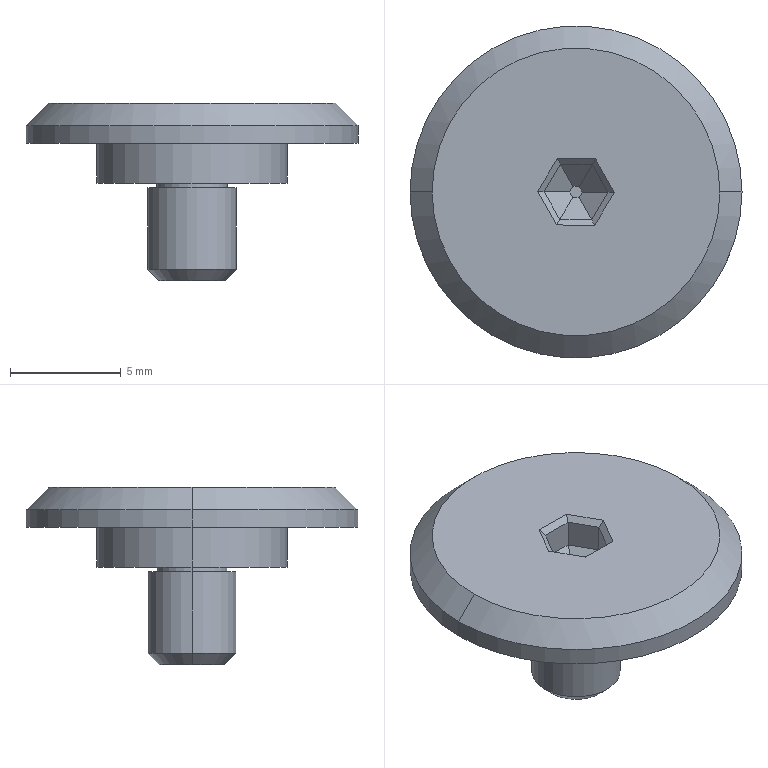Part | NX | features BREP 1 | 1 solid | 36 faces | box 15 x 15 x 8 mm | volume 442.432 mm3 | plane 24 | cylinder 8 | cone 4 | commonest cylinder face diameters 3.2 x2 4 x2 8.6 x2 15 x2
STEP:
#1=CARTESIAN_POINT('',(76.343,184.663,-5.));
#2=VERTEX_POINT('',#1);
#3=CARTESIAN_POINT('',(79.343,184.663,-5.));
#4=VERTEX_POINT('',#3);
#5=CARTESIAN_POINT('',(77.843,184.663,-5.));
#6=DIRECTION('',(0.,0.,-1.));
#7=DIRECTION('',(1.,0.,0.));
#8=AXIS2_PLACEMENT_3D('',#5,#6,#7);
#9=CIRCLE('',#8,1.5);
#10=EDGE_CURVE('',#2,#4,#9,.T.);
#11=ORIENTED_EDGE('',*,*,#10,.F.);
#12=CARTESIAN_POINT('',(75.843,184.663,-4.5));
#13=VERTEX_POINT('',#12);
#14=CARTESIAN_POINT('',(75.843,184.663,-4.5));
#15=DIRECTION('',(-0.7071,0.,0.7071));
#16=VECTOR('',#15,1000.);
#17=LINE('',#14,#16);
#18=EDGE_CURVE('',#2,#13,#17,.T.);
#19=ORIENTED_EDGE('',*,*,#18,.T.);
#20=CARTESIAN_POINT('',(79.843,184.663,-4.5));
#21=VERTEX_POINT('',#20);
#22=CARTESIAN_POINT('',(77.843,184.663,-4.5));
#23=DIRECTION('',(0.,0.,1.));
#24=DIRECTION('',(1.,0.,0.));
#25=AXIS2_PLACEMENT_3D('',#22,#23,#24);
#26=CIRCLE('',#25,2.);
#27=EDGE_CURVE('',#21,#13,#26,.T.);
#28=ORIENTED_EDGE('',*,*,#27,.F.);
#29=CARTESIAN_POINT('',(79.843,184.663,-4.5));
#30=DIRECTION('',(0.7071,0.,0.7071));
#31=VECTOR('',#30,1000.);
#32=LINE('',#29,#31);
#33=EDGE_CURVE('',#4,#21,#32,.T.);
#34=ORIENTED_EDGE('',*,*,#33,.F.);
#35=EDGE_LOOP('',(#11,#19,#28,#34));
#36=FACE_BOUND('',#35,.T.);
#37=CARTESIAN_POINT('',(77.843,184.663,-4.5));
#38=DIRECTION('',(0.,0.,1.));
#39=DIRECTION('',(-1.,0.,0.));
#40=AXIS2_PLACEMENT_3D('',#37,#38,#39);
#41=CONICAL_SURFACE('',#40,2.,0.7854);
#42=ADVANCED_FACE('',(#36),#41,.T.);
#43=ORIENTED_EDGE('',*,*,#27,.T.);
#44=CARTESIAN_POINT('',(75.843,184.663,-0.8));
#45=VERTEX_POINT('',#44);
#46=CARTESIAN_POINT('',(75.843,184.663,-4.));
#47=DIRECTION('',(0.,0.,1.));
#48=VECTOR('',#47,1000.);
#49=LINE('',#46,#48);
#50=EDGE_CURVE('',#13,#45,#49,.T.);
#51=ORIENTED_EDGE('',*,*,#50,.T.);
#52=CARTESIAN_POINT('',(79.843,184.663,-0.8));
#53=VERTEX_POINT('',#52);
#54=CARTESIAN_POINT('',(77.843,184.663,-0.8));
#55=DIRECTION('',(0.,0.,1.));
#56=DIRECTION('',(-1.,0.,0.));
#57=AXIS2_PLACEMENT_3D('',#54,#55,#56);
#58=CIRCLE('',#57,2.);
#59=EDGE_CURVE('',#53,#45,#58,.T.);
#60=ORIENTED_EDGE('',*,*,#59,.F.);
#61=CARTESIAN_POINT('',(79.843,184.663,-4.));
#62=DIRECTION('',(0.,0.,1.));
#63=VECTOR('',#62,1000.);
#64=LINE('',#61,#63);
#65=EDGE_CURVE('',#21,#53,#64,.T.);
#66=ORIENTED_EDGE('',*,*,#65,.F.);
#67=EDGE_LOOP('',(#43,#51,#60,#66));
#68=FACE_BOUND('',#67,.T.);
#69=CARTESIAN_POINT('',(77.843,184.663,-4.));
#70=DIRECTION('',(0.,0.,1.));
#71=DIRECTION('',(-1.,0.,0.));
#72=AXIS2_PLACEMENT_3D('',#69,#70,#71);
#73=CYLINDRICAL_SURFACE('',#72,2.);
#74=ADVANCED_FACE('',(#68),#73,.T.);
#75=CARTESIAN_POINT('',(76.243,184.663,-0.8));
#76=VERTEX_POINT('',#75);
#77=CARTESIAN_POINT('',(79.443,184.663,-0.8));
#78=VERTEX_POINT('',#77);
#79=CARTESIAN_POINT('',(77.843,184.663,-0.8));
#80=DIRECTION('',(0.,0.,-1.));
#81=DIRECTION('',(-1.,0.,0.));
#82=AXIS2_PLACEMENT_3D('',#79,#80,#81);
#83=CIRCLE('',#82,1.6);
#84=EDGE_CURVE('',#76,#78,#83,.T.);
#85=ORIENTED_EDGE('',*,*,#84,.F.);
#86=CARTESIAN_POINT('',(76.243,184.663,-0.6));
#87=VERTEX_POINT('',#86);
#88=CARTESIAN_POINT('',(76.243,184.663,-0.8));
#89=DIRECTION('',(0.,0.,1.));
#90=VECTOR('',#89,1000.);
#91=LINE('',#88,#90);
#92=EDGE_CURVE('',#76,#87,#91,.T.);
#93=ORIENTED_EDGE('',*,*,#92,.T.);
#94=CARTESIAN_POINT('',(79.443,184.663,-0.6));
#95=VERTEX_POINT('',#94);
#96=CARTESIAN_POINT('',(77.843,184.663,-0.6));
#97=DIRECTION('',(0.,0.,-1.));
#98=DIRECTION('',(1.,0.,0.));
#99=AXIS2_PLACEMENT_3D('',#96,#97,#98);
#100=CIRCLE('',#99,1.6);
#101=EDGE_CURVE('',#87,#95,#100,.T.);
#102=ORIENTED_EDGE('',*,*,#101,.T.);
#103=CARTESIAN_POINT('',(79.443,184.663,-0.8));
#104=DIRECTION('',(0.,0.,1.));
#105=VECTOR('',#104,1000.);
#106=LINE('',#103,#105);
#107=EDGE_CURVE('',#78,#95,#106,.T.);
#108=ORIENTED_EDGE('',*,*,#107,.F.);
#109=EDGE_LOOP('',(#85,#93,#102,#108));
#110=FACE_BOUND('',#109,.T.);
#111=CARTESIAN_POINT('',(77.843,184.663,-0.8));
#112=DIRECTION('',(0.,0.,1.));
#113=DIRECTION('',(-1.,0.,0.));
#114=AXIS2_PLACEMENT_3D('',#111,#112,#113);
#115=CYLINDRICAL_SURFACE('',#114,1.6);
#116=ADVANCED_FACE('',(#110),#115,.T.);
#117=CARTESIAN_POINT('',(84.343,184.663,3.));
#118=VERTEX_POINT('',#117);
#119=CARTESIAN_POINT('',(71.343,184.663,3.));
#120=VERTEX_POINT('',#119);
#121=CARTESIAN_POINT('',(77.843,184.663,3.));
#122=DIRECTION('',(0.,0.,1.));
#123=DIRECTION('',(1.,0.,0.));
#124=AXIS2_PLACEMENT_3D('',#121,#122,#123);
#125=CIRCLE('',#124,6.5);
#126=EDGE_CURVE('',#118,#120,#125,.T.);
#127=ORIENTED_EDGE('',*,*,#126,.F.);
#128=CARTESIAN_POINT('',(85.343,184.663,2.));
#129=VERTEX_POINT('',#128);
#130=CARTESIAN_POINT('',(84.343,184.663,3.));
#131=DIRECTION('',(0.7071,0.,-0.7071));
#132=VECTOR('',#131,1000.);
#133=LINE('',#130,#132);
#134=EDGE_CURVE('',#129,#118,#133,.F.);
#135=ORIENTED_EDGE('',*,*,#134,.F.);
#136=CARTESIAN_POINT('',(70.343,184.663,2.));
#137=VERTEX_POINT('',#136);
#138=CARTESIAN_POINT('',(77.843,184.663,2.));
#139=DIRECTION('',(0.,0.,-1.));
#140=DIRECTION('',(1.,0.,0.));
#141=AXIS2_PLACEMENT_3D('',#138,#139,#140);
#142=CIRCLE('',#141,7.5);
#143=EDGE_CURVE('',#137,#129,#142,.T.);
#144=ORIENTED_EDGE('',*,*,#143,.F.);
#145=CARTESIAN_POINT('',(71.343,184.663,3.));
#146=DIRECTION('',(-0.7071,0.,-0.7071));
#147=VECTOR('',#146,1000.);
#148=LINE('',#145,#147);
#149=EDGE_CURVE('',#137,#120,#148,.F.);
#150=ORIENTED_EDGE('',*,*,#149,.T.);
#151=EDGE_LOOP('',(#127,#135,#144,#150));
#152=FACE_BOUND('',#151,.T.);
#153=CARTESIAN_POINT('',(77.843,184.663,3.));
#154=DIRECTION('',(0.,0.,-1.));
#155=DIRECTION('',(1.,0.,0.));
#156=AXIS2_PLACEMENT_3D('',#153,#154,#155);
#157=CONICAL_SURFACE('',#156,6.5,0.7854);
#158=ADVANCED_FACE('',(#152),#157,.T.);
#159=ORIENTED_EDGE('',*,*,#143,.T.);
#160=CARTESIAN_POINT('',(85.343,184.663,1.2));
#161=VERTEX_POINT('',#160);
#162=CARTESIAN_POINT('',(85.343,184.663,2.));
#163=DIRECTION('',(0.,0.,-1.));
#164=VECTOR('',#163,1000.);
#165=LINE('',#162,#164);
#166=EDGE_CURVE('',#161,#129,#165,.F.);
#167=ORIENTED_EDGE('',*,*,#166,.F.);
#168=CARTESIAN_POINT('',(70.343,184.663,1.2));
#169=VERTEX_POINT('',#168);
#170=CARTESIAN_POINT('',(77.843,184.663,1.2));
#171=DIRECTION('',(0.,0.,1.));
#172=DIRECTION('',(1.,0.,0.));
#173=AXIS2_PLACEMENT_3D('',#170,#171,#172);
#174=CIRCLE('',#173,7.5);
#175=EDGE_CURVE('',#161,#169,#174,.T.);
#176=ORIENTED_EDGE('',*,*,#175,.T.);
#177=CARTESIAN_POINT('',(70.343,184.663,2.));
#178=DIRECTION('',(0.,0.,-1.));
#179=VECTOR('',#178,1000.);
#180=LINE('',#177,#179);
#181=EDGE_CURVE('',#169,#137,#180,.F.);
#182=ORIENTED_EDGE('',*,*,#181,.T.);
#183=EDGE_LOOP('',(#159,#167,#176,#182));
#184=FACE_BOUND('',#183,.T.);
#185=CARTESIAN_POINT('',(77.843,184.663,2.));
#186=DIRECTION('',(0.,0.,-1.));
#187=DIRECTION('',(1.,0.,0.));
#188=AXIS2_PLACEMENT_3D('',#185,#186,#187);
#189=CYLINDRICAL_SURFACE('',#188,7.5);
#190=ADVANCED_FACE('',(#184),#189,.T.);
#191=CARTESIAN_POINT('',(82.143,184.663,1.2));
#192=VERTEX_POINT('',#191);
#193=CARTESIAN_POINT('',(73.543,184.663,1.2));
#194=VERTEX_POINT('',#193);
#195=CARTESIAN_POINT('',(77.843,184.663,1.2));
#196=DIRECTION('',(0.,0.,1.));
#197=DIRECTION('',(1.,0.,0.));
#198=AXIS2_PLACEMENT_3D('',#195,#196,#197);
#199=CIRCLE('',#198,4.3);
#200=EDGE_CURVE('',#192,#194,#199,.T.);
#201=ORIENTED_EDGE('',*,*,#200,.F.);
#202=CARTESIAN_POINT('',(82.143,184.663,-0.6));
#203=VERTEX_POINT('',#202);
#204=CARTESIAN_POINT('',(82.143,184.663,1.));
#205=DIRECTION('',(0.,0.,-1.));
#206=VECTOR('',#205,1000.);
#207=LINE('',#204,#206);
#208=EDGE_CURVE('',#203,#192,#207,.F.);
#209=ORIENTED_EDGE('',*,*,#208,.F.);
#210=CARTESIAN_POINT('',(73.543,184.663,-0.6));
#211=VERTEX_POINT('',#210);
#212=CARTESIAN_POINT('',(77.843,184.663,-0.6));
#213=DIRECTION('',(0.,0.,1.));
#214=DIRECTION('',(1.,0.,0.));
#215=AXIS2_PLACEMENT_3D('',#212,#213,#214);
#216=CIRCLE('',#215,4.3);
#217=EDGE_CURVE('',#203,#211,#216,.T.);
#218=ORIENTED_EDGE('',*,*,#217,.T.);
#219=CARTESIAN_POINT('',(73.543,184.663,1.));
#220=DIRECTION('',(0.,0.,-1.));
#221=VECTOR('',#220,1000.);
#222=LINE('',#219,#221);
#223=EDGE_CURVE('',#211,#194,#222,.F.);
#224=ORIENTED_EDGE('',*,*,#223,.T.);
#225=EDGE_LOOP('',(#201,#209,#218,#224));
#226=FACE_BOUND('',#225,.T.);
#227=CARTESIAN_POINT('',(77.843,184.663,1.));
#228=DIRECTION('',(0.,0.,-1.));
#229=DIRECTION('',(1.,0.,0.));
#230=AXIS2_PLACEMENT_3D('',#227,#228,#229);
#231=CYLINDRICAL_SURFACE('',#230,4.3);
#232=ADVANCED_FACE('',(#226),#231,.T.);
#233=ORIENTED_EDGE('',*,*,#208,.T.);
#234=CARTESIAN_POINT('',(77.843,184.663,1.2));
#235=DIRECTION('',(0.,0.,1.));
#236=DIRECTION('',(1.,0.,0.));
#237=AXIS2_PLACEMENT_3D('',#234,#235,#236);
#238=CIRCLE('',#237,4.3);
#239=EDGE_CURVE('',#194,#192,#238,.T.);
#240=ORIENTED_EDGE('',*,*,#239,.F.);
#241=ORIENTED_EDGE('',*,*,#223,.F.);
#242=CARTESIAN_POINT('',(77.843,184.663,-0.6));
#243=DIRECTION('',(0.,0.,1.));
#244=DIRECTION('',(1.,0.,0.));
#245=AXIS2_PLACEMENT_3D('',#242,#243,#244);
#246=CIRCLE('',#245,4.3);
#247=EDGE_CURVE('',#211,#203,#246,.T.);
#248=ORIENTED_EDGE('',*,*,#247,.T.);
#249=EDGE_LOOP('',(#233,#240,#241,#248));
#250=FACE_BOUND('',#249,.T.);
#251=CARTESIAN_POINT('',(77.843,184.663,1.));
#252=DIRECTION('',(0.,0.,-1.));
#253=DIRECTION('',(1.,0.,0.));
#254=AXIS2_PLACEMENT_3D('',#251,#252,#253);
#255=CYLINDRICAL_SURFACE('',#254,4.3);
#256=ADVANCED_FACE('',(#250),#255,.T.);
#257=ORIENTED_EDGE('',*,*,#247,.F.);
#258=ORIENTED_EDGE('',*,*,#217,.F.);
#259=EDGE_LOOP('',(#257,#258));
#260=FACE_BOUND('',#259,.T.);
#261=CARTESIAN_POINT('',(77.843,184.663,-0.6));
#262=DIRECTION('',(0.,0.,-1.));
#263=DIRECTION('',(1.,0.,0.));
#264=AXIS2_PLACEMENT_3D('',#261,#262,#263);
#265=CIRCLE('',#264,1.6);
#266=EDGE_CURVE('',#95,#87,#265,.T.);
#267=ORIENTED_EDGE('',*,*,#266,.F.);
#268=ORIENTED_EDGE('',*,*,#101,.F.);
#269=EDGE_LOOP('',(#267,#268));
#270=FACE_BOUND('',#269,.T.);
#271=CARTESIAN_POINT('',(77.843,184.663,-0.6));
#272=DIRECTION('',(0.,0.,1.));
#273=DIRECTION('',(-1.,0.,0.));
#274=AXIS2_PLACEMENT_3D('',#271,#272,#273);
#275=PLANE('',#274);
#276=ADVANCED_FACE('',(#260,#270),#275,.F.);
#277=ORIENTED_EDGE('',*,*,#166,.T.);
#278=CARTESIAN_POINT('',(77.843,184.663,2.));
#279=DIRECTION('',(0.,0.,-1.));
#280=DIRECTION('',(1.,0.,0.));
#281=AXIS2_PLACEMENT_3D('',#278,#279,#280);
#282=CIRCLE('',#281,7.5);
#283=EDGE_CURVE('',#129,#137,#282,.T.);
#284=ORIENTED_EDGE('',*,*,#283,.T.);
#285=ORIENTED_EDGE('',*,*,#181,.F.);
#286=CARTESIAN_POINT('',(77.843,184.663,1.2));
#287=DIRECTION('',(0.,0.,1.));
#288=DIRECTION('',(1.,0.,0.));
#289=AXIS2_PLACEMENT_3D('',#286,#287,#288);
#290=CIRCLE('',#289,7.5);
#291=EDGE_CURVE('',#169,#161,#290,.T.);
#292=ORIENTED_EDGE('',*,*,#291,.T.);
#293=EDGE_LOOP('',(#277,#284,#285,#292));
#294=FACE_BOUND('',#293,.T.);
#295=CARTESIAN_POINT('',(77.843,184.663,2.));
#296=DIRECTION('',(0.,0.,-1.));
#297=DIRECTION('',(1.,0.,0.));
#298=AXIS2_PLACEMENT_3D('',#295,#296,#297);
#299=CYLINDRICAL_SURFACE('',#298,7.5);
#300=ADVANCED_FACE('',(#294),#299,.T.);
#301=CARTESIAN_POINT('',(77.843,184.663,3.));
#302=DIRECTION('',(0.,0.,1.));
#303=DIRECTION('',(1.,0.,0.));
#304=AXIS2_PLACEMENT_3D('',#301,#302,#303);
#305=CIRCLE('',#304,6.5);
#306=EDGE_CURVE('',#120,#118,#305,.T.);
#307=ORIENTED_EDGE('',*,*,#306,.T.);
#308=ORIENTED_EDGE('',*,*,#126,.T.);
#309=EDGE_LOOP('',(#307,#308));
#310=FACE_BOUND('',#309,.T.);
#311=CARTESIAN_POINT('',(76.111,184.683,3.));
#312=VERTEX_POINT('',#311);
#313=CARTESIAN_POINT('',(76.995,186.173,3.));
#314=VERTEX_POINT('',#313);
#315=CARTESIAN_POINT('',(76.921,186.049,3.));
#316=DIRECTION('',(0.5101,0.8601,0.));
#317=VECTOR('',#316,1000.);
#318=LINE('',#315,#317);
#319=EDGE_CURVE('',#312,#314,#318,.T.);
#320=ORIENTED_EDGE('',*,*,#319,.T.);
#321=CARTESIAN_POINT('',(78.727,186.152,3.));
#322=VERTEX_POINT('',#321);
#323=CARTESIAN_POINT('',(78.582,186.154,3.));
#324=DIRECTION('',(0.9999,-0.01175,0.));
#325=VECTOR('',#324,1000.);
#326=LINE('',#323,#325);
#327=EDGE_CURVE('',#314,#322,#326,.T.);
#328=ORIENTED_EDGE('',*,*,#327,.T.);
#329=CARTESIAN_POINT('',(79.575,184.642,3.));
#330=VERTEX_POINT('',#329);
#331=CARTESIAN_POINT('',(79.504,184.768,3.));
#332=DIRECTION('',(0.4898,-0.8718,0.));
#333=VECTOR('',#332,1000.);
#334=LINE('',#331,#333);
#335=EDGE_CURVE('',#322,#330,#334,.T.);
#336=ORIENTED_EDGE('',*,*,#335,.T.);
#337=CARTESIAN_POINT('',(78.691,183.153,3.));
#338=VERTEX_POINT('',#337);
#339=CARTESIAN_POINT('',(78.765,183.277,3.));
#340=DIRECTION('',(-0.5101,-0.8601,0.));
#341=VECTOR('',#340,1000.);
#342=LINE('',#339,#341);
#343=EDGE_CURVE('',#330,#338,#342,.T.);
#344=ORIENTED_EDGE('',*,*,#343,.T.);
#345=CARTESIAN_POINT('',(76.96,183.173,3.));
#346=VERTEX_POINT('',#345);
#347=CARTESIAN_POINT('',(77.104,183.171,3.));
#348=DIRECTION('',(-0.9999,0.01175,0.));
#349=VECTOR('',#348,1000.);
#350=LINE('',#347,#349);
#351=EDGE_CURVE('',#338,#346,#350,.T.);
#352=ORIENTED_EDGE('',*,*,#351,.T.);
#353=CARTESIAN_POINT('',(76.182,184.557,3.));
#354=DIRECTION('',(-0.4898,0.8718,0.));
#355=VECTOR('',#354,1000.);
#356=LINE('',#353,#355);
#357=EDGE_CURVE('',#346,#312,#356,.T.);
#358=ORIENTED_EDGE('',*,*,#357,.T.);
#359=EDGE_LOOP('',(#320,#328,#336,#344,#352,#358));
#360=FACE_BOUND('',#359,.T.);
#361=CARTESIAN_POINT('',(77.843,184.663,3.));
#362=DIRECTION('',(0.,0.,1.));
#363=DIRECTION('',(-1.,0.,0.));
#364=AXIS2_PLACEMENT_3D('',#361,#362,#363);
#365=PLANE('',#364);
#366=ADVANCED_FACE('',(#310,#360),#365,.T.);
#367=ORIENTED_EDGE('',*,*,#291,.F.);
#368=ORIENTED_EDGE('',*,*,#175,.F.);
#369=EDGE_LOOP('',(#367,#368));
#370=FACE_BOUND('',#369,.T.);
#371=ORIENTED_EDGE('',*,*,#239,.T.);
#372=ORIENTED_EDGE('',*,*,#200,.T.);
#373=EDGE_LOOP('',(#371,#372));
#374=FACE_BOUND('',#373,.T.);
#375=CARTESIAN_POINT('',(77.843,184.663,1.2));
#376=DIRECTION('',(0.,0.,1.));
#377=DIRECTION('',(-1.,0.,0.));
#378=AXIS2_PLACEMENT_3D('',#375,#376,#377);
#379=PLANE('',#378);
#380=ADVANCED_FACE('',(#370,#374),#379,.F.);
#381=CARTESIAN_POINT('',(79.286,184.646,1.5));
#382=VERTEX_POINT('',#381);
#383=CARTESIAN_POINT('',(79.286,184.646,2.75));
#384=VERTEX_POINT('',#383);
#385=CARTESIAN_POINT('',(79.286,184.646,1.5));
#386=DIRECTION('',(0.,0.,1.));
#387=VECTOR('',#386,1000.);
#388=LINE('',#385,#387);
#389=EDGE_CURVE('',#382,#384,#388,.T.);
#390=ORIENTED_EDGE('',*,*,#389,.T.);
#391=CARTESIAN_POINT('',(78.579,185.904,2.75));
#392=VERTEX_POINT('',#391);
#393=CARTESIAN_POINT('',(78.579,185.904,2.75));
#394=DIRECTION('',(-0.4898,0.8718,0.));
#395=VECTOR('',#394,1000.);
#396=LINE('',#393,#395);
#397=EDGE_CURVE('',#384,#392,#396,.T.);
#398=ORIENTED_EDGE('',*,*,#397,.T.);
#399=CARTESIAN_POINT('',(78.579,185.904,1.5));
#400=VERTEX_POINT('',#399);
#401=CARTESIAN_POINT('',(78.579,185.904,1.5));
#402=DIRECTION('',(0.,0.,1.));
#403=VECTOR('',#402,1000.);
#404=LINE('',#401,#403);
#405=EDGE_CURVE('',#400,#392,#404,.T.);
#406=ORIENTED_EDGE('',*,*,#405,.F.);
#407=CARTESIAN_POINT('',(79.286,184.646,1.5));
#408=DIRECTION('',(-0.4898,0.8718,0.));
#409=VECTOR('',#408,1000.);
#410=LINE('',#407,#409);
#411=EDGE_CURVE('',#382,#400,#410,.T.);
#412=ORIENTED_EDGE('',*,*,#411,.F.);
#413=EDGE_LOOP('',(#390,#398,#406,#412));
#414=FACE_BOUND('',#413,.T.);
#415=CARTESIAN_POINT('',(79.286,184.646,1.5));
#416=DIRECTION('',(0.8718,0.4898,0.));
#417=DIRECTION('',(0.,0.,1.));
#418=AXIS2_PLACEMENT_3D('',#415,#416,#417);
#419=PLANE('',#418);
#420=ADVANCED_FACE('',(#414),#419,.F.);
#421=CARTESIAN_POINT('',(78.55,183.404,1.5));
#422=VERTEX_POINT('',#421);
#423=CARTESIAN_POINT('',(78.55,183.404,2.75));
#424=VERTEX_POINT('',#423);
#425=CARTESIAN_POINT('',(78.55,183.404,1.5));
#426=DIRECTION('',(0.,0.,1.));
#427=VECTOR('',#426,1000.);
#428=LINE('',#425,#427);
#429=EDGE_CURVE('',#422,#424,#428,.T.);
#430=ORIENTED_EDGE('',*,*,#429,.T.);
#431=CARTESIAN_POINT('',(79.286,184.646,2.75));
#432=DIRECTION('',(0.5101,0.8601,0.));
#433=VECTOR('',#432,1000.);
#434=LINE('',#431,#433);
#435=EDGE_CURVE('',#424,#384,#434,.T.);
#436=ORIENTED_EDGE('',*,*,#435,.T.);
#437=ORIENTED_EDGE('',*,*,#389,.F.);
#438=CARTESIAN_POINT('',(78.55,183.404,1.5));
#439=DIRECTION('',(0.5101,0.8601,0.));
#440=VECTOR('',#439,1000.);
#441=LINE('',#438,#440);
#442=EDGE_CURVE('',#422,#382,#441,.T.);
#443=ORIENTED_EDGE('',*,*,#442,.F.);
#444=EDGE_LOOP('',(#430,#436,#437,#443));
#445=FACE_BOUND('',#444,.T.);
#446=CARTESIAN_POINT('',(78.55,183.404,1.5));
#447=DIRECTION('',(0.8601,-0.5101,0.));
#448=DIRECTION('',(0.,0.,1.));
#449=AXIS2_PLACEMENT_3D('',#446,#447,#448);
#450=PLANE('',#449);
#451=ADVANCED_FACE('',(#445),#450,.F.);
#452=CARTESIAN_POINT('',(77.107,183.421,1.5));
#453=VERTEX_POINT('',#452);
#454=CARTESIAN_POINT('',(77.107,183.421,2.75));
#455=VERTEX_POINT('',#454);
#456=CARTESIAN_POINT('',(77.107,183.421,1.5));
#457=DIRECTION('',(0.,0.,1.));
#458=VECTOR('',#457,1000.);
#459=LINE('',#456,#458);
#460=EDGE_CURVE('',#453,#455,#459,.T.);
#461=ORIENTED_EDGE('',*,*,#460,.T.);
#462=CARTESIAN_POINT('',(78.55,183.404,2.75));
#463=DIRECTION('',(0.9999,-0.01175,0.));
#464=VECTOR('',#463,1000.);
#465=LINE('',#462,#464);
#466=EDGE_CURVE('',#455,#424,#465,.T.);
#467=ORIENTED_EDGE('',*,*,#466,.T.);
#468=ORIENTED_EDGE('',*,*,#429,.F.);
#469=CARTESIAN_POINT('',(77.107,183.421,1.5));
#470=DIRECTION('',(0.9999,-0.01175,0.));
#471=VECTOR('',#470,1000.);
#472=LINE('',#469,#471);
#473=EDGE_CURVE('',#453,#422,#472,.T.);
#474=ORIENTED_EDGE('',*,*,#473,.F.);
#475=EDGE_LOOP('',(#461,#467,#468,#474));
#476=FACE_BOUND('',#475,.T.);
#477=CARTESIAN_POINT('',(77.107,183.421,1.5));
#478=DIRECTION('',(-0.01175,-0.9999,0.));
#479=DIRECTION('',(0.9999,-0.01175,0.));
#480=AXIS2_PLACEMENT_3D('',#477,#478,#479);
#481=PLANE('',#480);
#482=ADVANCED_FACE('',(#476),#481,.F.);
#483=CARTESIAN_POINT('',(76.4,184.68,1.5));
#484=VERTEX_POINT('',#483);
#485=CARTESIAN_POINT('',(76.4,184.68,2.75));
#486=VERTEX_POINT('',#485);
#487=CARTESIAN_POINT('',(76.4,184.68,1.5));
#488=DIRECTION('',(0.,0.,1.));
#489=VECTOR('',#488,1000.);
#490=LINE('',#487,#489);
#491=EDGE_CURVE('',#484,#486,#490,.T.);
#492=ORIENTED_EDGE('',*,*,#491,.T.);
#493=CARTESIAN_POINT('',(77.107,183.421,2.75));
#494=DIRECTION('',(0.4898,-0.8718,0.));
#495=VECTOR('',#494,1000.);
#496=LINE('',#493,#495);
#497=EDGE_CURVE('',#486,#455,#496,.T.);
#498=ORIENTED_EDGE('',*,*,#497,.T.);
#499=ORIENTED_EDGE('',*,*,#460,.F.);
#500=CARTESIAN_POINT('',(76.4,184.68,1.5));
#501=DIRECTION('',(0.4898,-0.8718,0.));
#502=VECTOR('',#501,1000.);
#503=LINE('',#500,#502);
#504=EDGE_CURVE('',#484,#453,#503,.T.);
#505=ORIENTED_EDGE('',*,*,#504,.F.);
#506=EDGE_LOOP('',(#492,#498,#499,#505));
#507=FACE_BOUND('',#506,.T.);
#508=CARTESIAN_POINT('',(76.4,184.68,1.5));
#509=DIRECTION('',(-0.8718,-0.4898,0.));
#510=DIRECTION('',(0.4898,-0.8718,0.));
#511=AXIS2_PLACEMENT_3D('',#508,#509,#510);
#512=PLANE('',#511);
#513=ADVANCED_FACE('',(#507),#512,.F.);
#514=CARTESIAN_POINT('',(77.136,185.921,1.5));
#515=VERTEX_POINT('',#514);
#516=CARTESIAN_POINT('',(77.136,185.921,2.75));
#517=VERTEX_POINT('',#516);
#518=CARTESIAN_POINT('',(77.136,185.921,1.5));
#519=DIRECTION('',(0.,0.,1.));
#520=VECTOR('',#519,1000.);
#521=LINE('',#518,#520);
#522=EDGE_CURVE('',#515,#517,#521,.T.);
#523=ORIENTED_EDGE('',*,*,#522,.T.);
#524=CARTESIAN_POINT('',(76.4,184.68,2.75));
#525=DIRECTION('',(-0.5101,-0.8601,0.));
#526=VECTOR('',#525,1000.);
#527=LINE('',#524,#526);
#528=EDGE_CURVE('',#517,#486,#527,.T.);
#529=ORIENTED_EDGE('',*,*,#528,.T.);
#530=ORIENTED_EDGE('',*,*,#491,.F.);
#531=CARTESIAN_POINT('',(77.136,185.921,1.5));
#532=DIRECTION('',(-0.5101,-0.8601,0.));
#533=VECTOR('',#532,1000.);
#534=LINE('',#531,#533);
#535=EDGE_CURVE('',#515,#484,#534,.T.);
#536=ORIENTED_EDGE('',*,*,#535,.F.);
#537=EDGE_LOOP('',(#523,#529,#530,#536));
#538=FACE_BOUND('',#537,.T.);
#539=CARTESIAN_POINT('',(77.136,185.921,1.5));
#540=DIRECTION('',(-0.8601,0.5101,0.));
#541=DIRECTION('',(0.,0.,-1.));
#542=AXIS2_PLACEMENT_3D('',#539,#540,#541);
#543=PLANE('',#542);
#544=ADVANCED_FACE('',(#538),#543,.F.);
#545=ORIENTED_EDGE('',*,*,#405,.T.);
#546=CARTESIAN_POINT('',(77.136,185.921,2.75));
#547=DIRECTION('',(-0.9999,0.01175,0.));
#548=VECTOR('',#547,1000.);
#549=LINE('',#546,#548);
#550=EDGE_CURVE('',#392,#517,#549,.T.);
#551=ORIENTED_EDGE('',*,*,#550,.T.);
#552=ORIENTED_EDGE('',*,*,#522,.F.);
#553=CARTESIAN_POINT('',(78.579,185.904,1.5));
#554=DIRECTION('',(-0.9999,0.01175,0.));
#555=VECTOR('',#554,1000.);
#556=LINE('',#553,#555);
#557=EDGE_CURVE('',#400,#515,#556,.T.);
#558=ORIENTED_EDGE('',*,*,#557,.F.);
#559=EDGE_LOOP('',(#545,#551,#552,#558));
#560=FACE_BOUND('',#559,.T.);
#561=CARTESIAN_POINT('',(78.579,185.904,1.5));
#562=DIRECTION('',(0.01175,0.9999,0.));
#563=DIRECTION('',(0.,0.,1.));
#564=AXIS2_PLACEMENT_3D('',#561,#562,#563);
#565=PLANE('',#564);
#566=ADVANCED_FACE('',(#560),#565,.F.);
#567=ORIENTED_EDGE('',*,*,#442,.T.);
#568=CARTESIAN_POINT('',(78.132,184.659,0.5));
#569=VERTEX_POINT('',#568);
#570=CARTESIAN_POINT('',(78.874,184.651,1.143));
#571=DIRECTION('',(0.7559,-0.008884,0.6547));
#572=VECTOR('',#571,1000.);
#573=LINE('',#570,#572);
#574=EDGE_CURVE('',#569,#382,#573,.T.);
#575=ORIENTED_EDGE('',*,*,#574,.F.);
#576=CARTESIAN_POINT('',(77.984,184.411,0.5));
#577=VERTEX_POINT('',#576);
#578=CARTESIAN_POINT('',(-23.225,13.775,0.5));
#579=DIRECTION('',(0.5101,0.8601,0.));
#580=VECTOR('',#579,1000.);
#581=LINE('',#578,#580);
#582=EDGE_CURVE('',#577,#569,#581,.T.);
#583=ORIENTED_EDGE('',*,*,#582,.F.);
#584=CARTESIAN_POINT('',(78.348,183.764,1.143));
#585=DIRECTION('',(0.3702,-0.6591,0.6547));
#586=VECTOR('',#585,1000.);
#587=LINE('',#584,#586);
#588=EDGE_CURVE('',#577,#422,#587,.T.);
#589=ORIENTED_EDGE('',*,*,#588,.T.);
#590=EDGE_LOOP('',(#567,#575,#583,#589));
#591=FACE_BOUND('',#590,.T.);
#592=CARTESIAN_POINT('',(78.55,183.404,1.5));
#593=DIRECTION('',(0.6082,-0.3607,-0.7071));
#594=DIRECTION('',(0.,0.8908,-0.4544));
#595=AXIS2_PLACEMENT_3D('',#592,#593,#594);
#596=PLANE('',#595);
#597=ADVANCED_FACE('',(#591),#596,.F.);
#598=ORIENTED_EDGE('',*,*,#473,.T.);
#599=ORIENTED_EDGE('',*,*,#588,.F.);
#600=CARTESIAN_POINT('',(77.696,184.414,0.5));
#601=VERTEX_POINT('',#600);
#602=CARTESIAN_POINT('',(2.178,185.302,0.5));
#603=DIRECTION('',(0.9999,-0.01175,0.));
#604=VECTOR('',#603,1000.);
#605=LINE('',#602,#604);
#606=EDGE_CURVE('',#601,#577,#605,.T.);
#607=ORIENTED_EDGE('',*,*,#606,.F.);
#608=CARTESIAN_POINT('',(77.317,183.776,1.143));
#609=DIRECTION('',(-0.3856,-0.6502,0.6547));
#610=VECTOR('',#609,1000.);
#611=LINE('',#608,#610);
#612=EDGE_CURVE('',#601,#453,#611,.T.);
#613=ORIENTED_EDGE('',*,*,#612,.T.);
#614=EDGE_LOOP('',(#598,#599,#607,#613));
#615=FACE_BOUND('',#614,.T.);
#616=CARTESIAN_POINT('',(77.107,183.421,1.5));
#617=DIRECTION('',(-0.008311,-0.7071,-0.7071));
#618=DIRECTION('',(0.,0.7071,-0.7071));
#619=AXIS2_PLACEMENT_3D('',#616,#617,#618);
#620=PLANE('',#619);
#621=ADVANCED_FACE('',(#615),#620,.F.);
#622=ORIENTED_EDGE('',*,*,#504,.T.);
#623=ORIENTED_EDGE('',*,*,#612,.F.);
#624=CARTESIAN_POINT('',(77.554,184.666,0.5));
#625=VERTEX_POINT('',#624);
#626=CARTESIAN_POINT('',(137.805,77.417,0.5));
#627=DIRECTION('',(0.4898,-0.8718,0.));
#628=VECTOR('',#627,1000.);
#629=LINE('',#626,#628);
#630=EDGE_CURVE('',#625,#601,#629,.T.);
#631=ORIENTED_EDGE('',*,*,#630,.F.);
#632=CARTESIAN_POINT('',(76.812,184.675,1.143));
#633=DIRECTION('',(-0.7559,0.008884,0.6547));
#634=VECTOR('',#633,1000.);
#635=LINE('',#632,#634);
#636=EDGE_CURVE('',#625,#484,#635,.T.);
#637=ORIENTED_EDGE('',*,*,#636,.T.);
#638=EDGE_LOOP('',(#622,#623,#631,#637));
#639=FACE_BOUND('',#638,.T.);
#640=CARTESIAN_POINT('',(76.4,184.68,1.5));
#641=DIRECTION('',(-0.6165,-0.3463,-0.7071));
#642=DIRECTION('',(0.7538,0.,-0.6572));
#643=AXIS2_PLACEMENT_3D('',#640,#641,#642);
#644=PLANE('',#643);
#645=ADVANCED_FACE('',(#639),#644,.F.);
#646=ORIENTED_EDGE('',*,*,#535,.T.);
#647=ORIENTED_EDGE('',*,*,#636,.F.);
#648=CARTESIAN_POINT('',(77.702,184.914,0.5));
#649=VERTEX_POINT('',#648);
#650=CARTESIAN_POINT('',(-23.655,14.03,0.5));
#651=DIRECTION('',(-0.5101,-0.8601,0.));
#652=VECTOR('',#651,1000.);
#653=LINE('',#650,#652);
#654=EDGE_CURVE('',#649,#625,#653,.T.);
#655=ORIENTED_EDGE('',*,*,#654,.F.);
#656=CARTESIAN_POINT('',(77.338,185.562,1.143));
#657=DIRECTION('',(-0.3702,0.6591,0.6547));
#658=VECTOR('',#657,1000.);
#659=LINE('',#656,#658);
#660=EDGE_CURVE('',#649,#515,#659,.T.);
#661=ORIENTED_EDGE('',*,*,#660,.T.);
#662=EDGE_LOOP('',(#646,#647,#655,#661));
#663=FACE_BOUND('',#662,.T.);
#664=CARTESIAN_POINT('',(77.136,185.921,1.5));
#665=DIRECTION('',(-0.6082,0.3607,-0.7071));
#666=DIRECTION('',(0.7582,0.,-0.6521));
#667=AXIS2_PLACEMENT_3D('',#664,#665,#666);
#668=PLANE('',#667);
#669=ADVANCED_FACE('',(#663),#668,.F.);
#670=ORIENTED_EDGE('',*,*,#557,.T.);
#671=ORIENTED_EDGE('',*,*,#660,.F.);
#672=CARTESIAN_POINT('',(77.99,184.911,0.5));
#673=VERTEX_POINT('',#672);
#674=CARTESIAN_POINT('',(2.184,185.802,0.5));
#675=DIRECTION('',(-0.9999,0.01175,0.));
#676=VECTOR('',#675,1000.);
#677=LINE('',#674,#676);
#678=EDGE_CURVE('',#673,#649,#677,.T.);
#679=ORIENTED_EDGE('',*,*,#678,.F.);
#680=CARTESIAN_POINT('',(78.369,185.549,1.143));
#681=DIRECTION('',(0.3856,0.6502,0.6547));
#682=VECTOR('',#681,1000.);
#683=LINE('',#680,#682);
#684=EDGE_CURVE('',#673,#400,#683,.T.);
#685=ORIENTED_EDGE('',*,*,#684,.T.);
#686=EDGE_LOOP('',(#670,#671,#679,#685));
#687=FACE_BOUND('',#686,.T.);
#688=CARTESIAN_POINT('',(78.579,185.904,1.5));
#689=DIRECTION('',(0.008311,0.7071,-0.7071));
#690=DIRECTION('',(0.9999,0.,0.01175));
#691=AXIS2_PLACEMENT_3D('',#688,#689,#690);
#692=PLANE('',#691);
#693=ADVANCED_FACE('',(#687),#692,.F.);
#694=ORIENTED_EDGE('',*,*,#411,.T.);
#695=ORIENTED_EDGE('',*,*,#684,.F.);
#696=CARTESIAN_POINT('',(138.241,77.662,0.5));
#697=DIRECTION('',(-0.4898,0.8718,0.));
#698=VECTOR('',#697,1000.);
#699=LINE('',#696,#698);
#700=EDGE_CURVE('',#569,#673,#699,.T.);
#701=ORIENTED_EDGE('',*,*,#700,.F.);
#702=ORIENTED_EDGE('',*,*,#574,.T.);
#703=EDGE_LOOP('',(#694,#695,#701,#702));
#704=FACE_BOUND('',#703,.T.);
#705=CARTESIAN_POINT('',(79.286,184.646,1.5));
#706=DIRECTION('',(0.6165,0.3463,-0.7071));
#707=DIRECTION('',(0.,0.8981,0.4399));
#708=AXIS2_PLACEMENT_3D('',#705,#706,#707);
#709=PLANE('',#708);
#710=ADVANCED_FACE('',(#704),#709,.F.);
#711=ORIENTED_EDGE('',*,*,#582,.T.);
#712=ORIENTED_EDGE('',*,*,#700,.T.);
#713=ORIENTED_EDGE('',*,*,#678,.T.);
#714=ORIENTED_EDGE('',*,*,#654,.T.);
#715=ORIENTED_EDGE('',*,*,#630,.T.);
#716=ORIENTED_EDGE('',*,*,#606,.T.);
#717=EDGE_LOOP('',(#711,#712,#713,#714,#715,#716));
#718=FACE_BOUND('',#717,.T.);
#719=CARTESIAN_POINT('',(0.,0.,0.5));
#720=DIRECTION('',(0.,0.,1.));
#721=DIRECTION('',(-1.,0.,0.));
#722=AXIS2_PLACEMENT_3D('',#719,#720,#721);
#723=PLANE('',#722);
#724=ADVANCED_FACE('',(#718),#723,.T.);
#725=CARTESIAN_POINT('',(77.317,183.776,2.393));
#726=DIRECTION('',(0.3856,0.6502,-0.6547));
#727=VECTOR('',#726,1000.);
#728=LINE('',#725,#727);
#729=EDGE_CURVE('',#346,#455,#728,.T.);
#730=ORIENTED_EDGE('',*,*,#729,.F.);
#731=ORIENTED_EDGE('',*,*,#351,.F.);
#732=CARTESIAN_POINT('',(78.348,183.764,2.393));
#733=DIRECTION('',(0.3702,-0.6591,0.6547));
#734=VECTOR('',#733,1000.);
#735=LINE('',#732,#734);
#736=EDGE_CURVE('',#424,#338,#735,.T.);
#737=ORIENTED_EDGE('',*,*,#736,.F.);
#738=ORIENTED_EDGE('',*,*,#466,.F.);
#739=EDGE_LOOP('',(#730,#731,#737,#738));
#740=FACE_BOUND('',#739,.T.);
#741=CARTESIAN_POINT('',(77.107,183.421,2.75));
#742=DIRECTION('',(0.008311,0.7071,0.7071));
#743=DIRECTION('',(-0.9999,0.01175,0.));
#744=AXIS2_PLACEMENT_3D('',#741,#742,#743);
#745=PLANE('',#744);
#746=ADVANCED_FACE('',(#740),#745,.T.);
#747=ORIENTED_EDGE('',*,*,#736,.T.);
#748=ORIENTED_EDGE('',*,*,#343,.F.);
#749=CARTESIAN_POINT('',(78.874,184.651,2.393));
#750=DIRECTION('',(0.7559,-0.008884,0.6547));
#751=VECTOR('',#750,1000.);
#752=LINE('',#749,#751);
#753=EDGE_CURVE('',#384,#330,#752,.T.);
#754=ORIENTED_EDGE('',*,*,#753,.F.);
#755=ORIENTED_EDGE('',*,*,#435,.F.);
#756=EDGE_LOOP('',(#747,#748,#754,#755));
#757=FACE_BOUND('',#756,.T.);
#758=CARTESIAN_POINT('',(78.55,183.404,2.75));
#759=DIRECTION('',(-0.6082,0.3607,0.7071));
#760=DIRECTION('',(-0.5101,-0.8601,0.));
#761=AXIS2_PLACEMENT_3D('',#758,#759,#760);
#762=PLANE('',#761);
#763=ADVANCED_FACE('',(#757),#762,.T.);
#764=ORIENTED_EDGE('',*,*,#729,.T.);
#765=ORIENTED_EDGE('',*,*,#497,.F.);
#766=CARTESIAN_POINT('',(76.812,184.675,2.393));
#767=DIRECTION('',(0.7559,-0.008884,-0.6547));
#768=VECTOR('',#767,1000.);
#769=LINE('',#766,#768);
#770=EDGE_CURVE('',#312,#486,#769,.T.);
#771=ORIENTED_EDGE('',*,*,#770,.F.);
#772=ORIENTED_EDGE('',*,*,#357,.F.);
#773=EDGE_LOOP('',(#764,#765,#771,#772));
#774=FACE_BOUND('',#773,.T.);
#775=CARTESIAN_POINT('',(76.4,184.68,2.75));
#776=DIRECTION('',(0.6165,0.3463,0.7071));
#777=DIRECTION('',(-0.4898,0.8718,0.));
#778=AXIS2_PLACEMENT_3D('',#775,#776,#777);
#779=PLANE('',#778);
#780=ADVANCED_FACE('',(#774),#779,.T.);
#781=ORIENTED_EDGE('',*,*,#753,.T.);
#782=ORIENTED_EDGE('',*,*,#335,.F.);
#783=CARTESIAN_POINT('',(78.579,185.904,2.75));
#784=DIRECTION('',(0.3856,0.6502,0.6547));
#785=VECTOR('',#784,1000.);
#786=LINE('',#783,#785);
#787=EDGE_CURVE('',#392,#322,#786,.T.);
#788=ORIENTED_EDGE('',*,*,#787,.F.);
#789=ORIENTED_EDGE('',*,*,#397,.F.);
#790=EDGE_LOOP('',(#781,#782,#788,#789));
#791=FACE_BOUND('',#790,.T.);
#792=CARTESIAN_POINT('',(79.286,184.646,2.75));
#793=DIRECTION('',(-0.6165,-0.3463,0.7071));
#794=DIRECTION('',(0.4898,-0.8718,0.));
#795=AXIS2_PLACEMENT_3D('',#792,#793,#794);
#796=PLANE('',#795);
#797=ADVANCED_FACE('',(#791),#796,.T.);
#798=ORIENTED_EDGE('',*,*,#770,.T.);
#799=ORIENTED_EDGE('',*,*,#528,.F.);
#800=CARTESIAN_POINT('',(77.338,185.562,2.393));
#801=DIRECTION('',(0.3702,-0.6591,-0.6547));
#802=VECTOR('',#801,1000.);
#803=LINE('',#800,#802);
#804=EDGE_CURVE('',#314,#517,#803,.T.);
#805=ORIENTED_EDGE('',*,*,#804,.F.);
#806=ORIENTED_EDGE('',*,*,#319,.F.);
#807=EDGE_LOOP('',(#798,#799,#805,#806));
#808=FACE_BOUND('',#807,.T.);
#809=CARTESIAN_POINT('',(77.136,185.921,2.75));
#810=DIRECTION('',(0.6082,-0.3607,0.7071));
#811=DIRECTION('',(0.5101,0.8601,0.));
#812=AXIS2_PLACEMENT_3D('',#809,#810,#811);
#813=PLANE('',#812);
#814=ADVANCED_FACE('',(#808),#813,.T.);
#815=ORIENTED_EDGE('',*,*,#787,.T.);
#816=ORIENTED_EDGE('',*,*,#327,.F.);
#817=ORIENTED_EDGE('',*,*,#804,.T.);
#818=ORIENTED_EDGE('',*,*,#550,.F.);
#819=EDGE_LOOP('',(#815,#816,#817,#818));
#820=FACE_BOUND('',#819,.T.);
#821=CARTESIAN_POINT('',(78.579,185.904,2.75));
#822=DIRECTION('',(-0.008311,-0.7071,0.7071));
#823=DIRECTION('',(0.9999,-0.01175,0.));
#824=AXIS2_PLACEMENT_3D('',#821,#822,#823);
#825=PLANE('',#824);
#826=ADVANCED_FACE('',(#820),#825,.T.);
#827=ORIENTED_EDGE('',*,*,#134,.T.);
#828=ORIENTED_EDGE('',*,*,#306,.F.);
#829=ORIENTED_EDGE('',*,*,#149,.F.);
#830=ORIENTED_EDGE('',*,*,#283,.F.);
#831=EDGE_LOOP('',(#827,#828,#829,#830));
#832=FACE_BOUND('',#831,.T.);
#833=CARTESIAN_POINT('',(77.843,184.663,3.));
#834=DIRECTION('',(0.,0.,-1.));
#835=DIRECTION('',(1.,0.,0.));
#836=AXIS2_PLACEMENT_3D('',#833,#834,#835);
#837=CONICAL_SURFACE('',#836,6.5,0.7854);
#838=ADVANCED_FACE('',(#832),#837,.T.);
#839=ORIENTED_EDGE('',*,*,#59,.T.);
#840=CARTESIAN_POINT('',(77.843,184.663,-0.8));
#841=DIRECTION('',(0.,0.,1.));
#842=DIRECTION('',(-1.,0.,0.));
#843=AXIS2_PLACEMENT_3D('',#840,#841,#842);
#844=CIRCLE('',#843,2.);
#845=EDGE_CURVE('',#45,#53,#844,.T.);
#846=ORIENTED_EDGE('',*,*,#845,.T.);
#847=EDGE_LOOP('',(#839,#846));
#848=FACE_BOUND('',#847,.T.);
#849=CARTESIAN_POINT('',(77.843,184.663,-0.8));
#850=DIRECTION('',(0.,0.,-1.));
#851=DIRECTION('',(-1.,0.,0.));
#852=AXIS2_PLACEMENT_3D('',#849,#850,#851);
#853=CIRCLE('',#852,1.6);
#854=EDGE_CURVE('',#78,#76,#853,.T.);
#855=ORIENTED_EDGE('',*,*,#854,.T.);
#856=ORIENTED_EDGE('',*,*,#84,.T.);
#857=EDGE_LOOP('',(#855,#856));
#858=FACE_BOUND('',#857,.T.);
#859=CARTESIAN_POINT('',(77.843,184.663,-0.8));
#860=DIRECTION('',(0.,0.,-1.));
#861=DIRECTION('',(0.,1.,0.));
#862=AXIS2_PLACEMENT_3D('',#859,#860,#861);
#863=PLANE('',#862);
#864=ADVANCED_FACE('',(#848,#858),#863,.F.);
#865=ORIENTED_EDGE('',*,*,#92,.F.);
#866=ORIENTED_EDGE('',*,*,#854,.F.);
#867=ORIENTED_EDGE('',*,*,#107,.T.);
#868=ORIENTED_EDGE('',*,*,#266,.T.);
#869=EDGE_LOOP('',(#865,#866,#867,#868));
#870=FACE_BOUND('',#869,.T.);
#871=CARTESIAN_POINT('',(77.843,184.663,-0.8));
#872=DIRECTION('',(0.,0.,1.));
#873=DIRECTION('',(-1.,0.,0.));
#874=AXIS2_PLACEMENT_3D('',#871,#872,#873);
#875=CYLINDRICAL_SURFACE('',#874,1.6);
#876=ADVANCED_FACE('',(#870),#875,.T.);
#877=CARTESIAN_POINT('',(77.843,184.663,-5.));
#878=DIRECTION('',(0.,0.,-1.));
#879=DIRECTION('',(1.,0.,0.));
#880=AXIS2_PLACEMENT_3D('',#877,#878,#879);
#881=CIRCLE('',#880,1.5);
#882=EDGE_CURVE('',#4,#2,#881,.T.);
#883=ORIENTED_EDGE('',*,*,#882,.T.);
#884=ORIENTED_EDGE('',*,*,#10,.T.);
#885=EDGE_LOOP('',(#883,#884));
#886=FACE_BOUND('',#885,.T.);
#887=CARTESIAN_POINT('',(77.843,184.663,-5.));
#888=DIRECTION('',(0.,0.,1.));
#889=DIRECTION('',(-1.,0.,0.));
#890=AXIS2_PLACEMENT_3D('',#887,#888,#889);
#891=PLANE('',#890);
#892=ADVANCED_FACE('',(#886),#891,.F.);
#893=ORIENTED_EDGE('',*,*,#50,.F.);
#894=CARTESIAN_POINT('',(77.843,184.663,-4.5));
#895=DIRECTION('',(0.,0.,1.));
#896=DIRECTION('',(1.,0.,0.));
#897=AXIS2_PLACEMENT_3D('',#894,#895,#896);
#898=CIRCLE('',#897,2.);
#899=EDGE_CURVE('',#13,#21,#898,.T.);
#900=ORIENTED_EDGE('',*,*,#899,.T.);
#901=ORIENTED_EDGE('',*,*,#65,.T.);
#902=ORIENTED_EDGE('',*,*,#845,.F.);
#903=EDGE_LOOP('',(#893,#900,#901,#902));
#904=FACE_BOUND('',#903,.T.);
#905=CARTESIAN_POINT('',(77.843,184.663,-4.));
#906=DIRECTION('',(0.,0.,1.));
#907=DIRECTION('',(-1.,0.,0.));
#908=AXIS2_PLACEMENT_3D('',#905,#906,#907);
#909=CYLINDRICAL_SURFACE('',#908,2.);
#910=ADVANCED_FACE('',(#904),#909,.T.);
#911=ORIENTED_EDGE('',*,*,#18,.F.);
#912=ORIENTED_EDGE('',*,*,#882,.F.);
#913=ORIENTED_EDGE('',*,*,#33,.T.);
#914=ORIENTED_EDGE('',*,*,#899,.F.);
#915=EDGE_LOOP('',(#911,#912,#913,#914));
#916=FACE_BOUND('',#915,.T.);
#917=CARTESIAN_POINT('',(77.843,184.663,-4.5));
#918=DIRECTION('',(0.,0.,1.));
#919=DIRECTION('',(-1.,0.,0.));
#920=AXIS2_PLACEMENT_3D('',#917,#918,#919);
#921=CONICAL_SURFACE('',#920,2.,0.7854);
#922=ADVANCED_FACE('',(#916),#921,.T.);
#923=CLOSED_SHELL('',(#42,#74,#116,#158,#190,#232,#256,#276,#300,#366,#380,#420,#451,#482,#513,#544,#566,#597,#621,#645,#669,#693,#710,#724,#746,#763,#780,#797,#814,#826,#838,#864,#876,#892,#910,#922));
#924=MANIFOLD_SOLID_BREP('',#923);
#925=(LENGTH_UNIT()NAMED_UNIT(*)SI_UNIT(.MILLI.,.METRE.));
#926=UNCERTAINTY_MEASURE_WITH_UNIT(LENGTH_MEASURE(0.00001),#925,'','');
#927=(NAMED_UNIT(*)PLANE_ANGLE_UNIT()SI_UNIT($,.RADIAN.));
#928=(NAMED_UNIT(*)SI_UNIT($,.STERADIAN.)SOLID_ANGLE_UNIT());
#929=(GEOMETRIC_REPRESENTATION_CONTEXT(3)GLOBAL_UNCERTAINTY_ASSIGNED_CONTEXT((#926))GLOBAL_UNIT_ASSIGNED_CONTEXT((#925,#927,#928))REPRESENTATION_CONTEXT('',''));
#930=ADVANCED_BREP_SHAPE_REPRESENTATION('',(#924),#929);